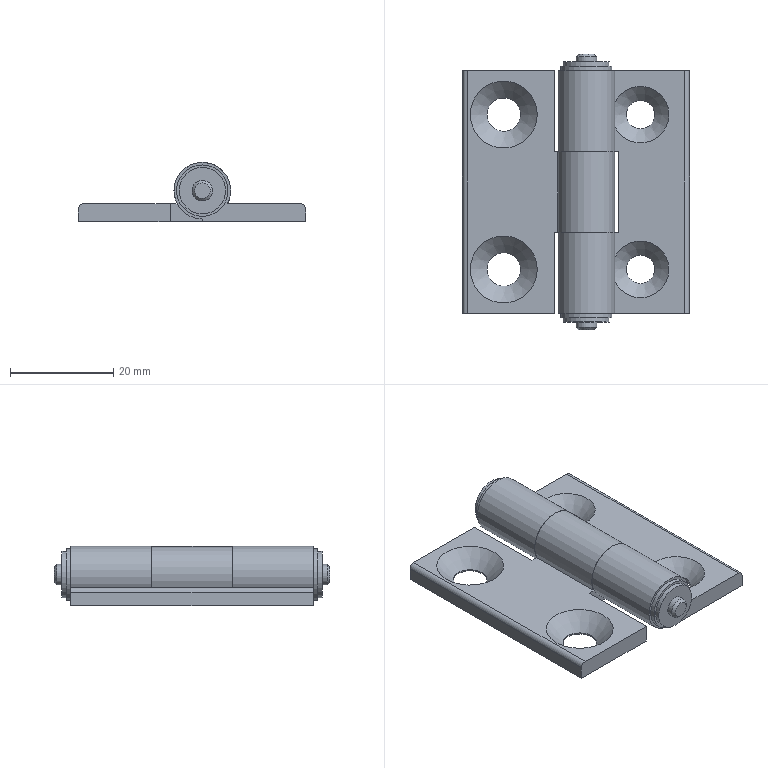Part | STEP file | C-HHFLS6-5 | 3 solids | 49 faces | box 44 x 53.4 x 11.5 mm | volume 9579 mm3 | plane 26 | cylinder 17 | cone 6 | commonest cylinder face diameters 4 x4 11 x3 2 x2 5.5 x2 6.5 x2 9 x2